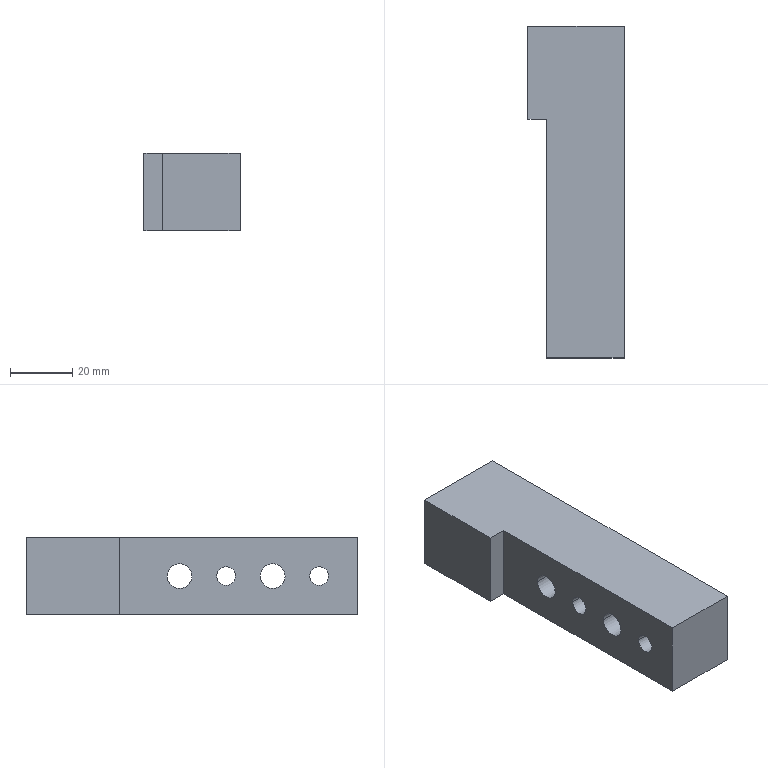Part | STEP file | Positioning_id1290_x_t | 1 solid | 16 faces | box 30.998 x 106.963 x 25 mm | volume 67424 mm3 | cylinder 8 | plane 8 | commonest cylinder face diameters 6 x4 8 x4